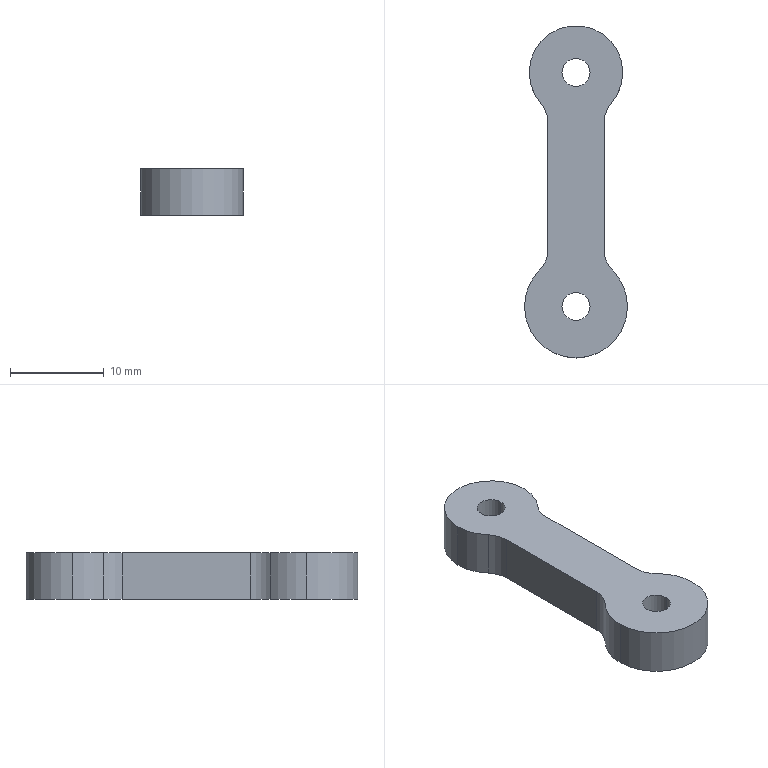Part | SolidWorks | features BaseBody 1 | 1 solid | 18 faces | box 11 x 35.5 x 5 mm | volume 1255 mm3 | cylinder 14 | plane 4 | commonest cylinder face diameters 3 x4 6 x4 10 x3 11 x3
STEP:
#1=CARTESIAN_POINT('',(1.5,25.,5.));
#2=VERTEX_POINT('',#1);
#3=CARTESIAN_POINT('',(1.5,25.,0.));
#4=VERTEX_POINT('',#3);
#5=CARTESIAN_POINT('',(1.5,25.,5.));
#6=DIRECTION('',(0.,0.,-1.));
#7=VECTOR('',#6,1000.);
#8=LINE('',#5,#7);
#9=EDGE_CURVE('',#2,#4,#8,.T.);
#10=ORIENTED_EDGE('',*,*,#9,.F.);
#11=CARTESIAN_POINT('',(-1.5,25.,5.));
#12=VERTEX_POINT('',#11);
#13=CARTESIAN_POINT('',(0.,25.,5.));
#14=DIRECTION('',(0.,0.,1.));
#15=DIRECTION('',(1.,0.,0.));
#16=AXIS2_PLACEMENT_3D('',#13,#14,#15);
#17=CIRCLE('',#16,1.5);
#18=EDGE_CURVE('',#2,#12,#17,.T.);
#19=ORIENTED_EDGE('',*,*,#18,.T.);
#20=CARTESIAN_POINT('',(-1.5,25.,0.));
#21=VERTEX_POINT('',#20);
#22=CARTESIAN_POINT('',(-1.5,25.,5.));
#23=DIRECTION('',(0.,0.,-1.));
#24=VECTOR('',#23,1000.);
#25=LINE('',#22,#24);
#26=EDGE_CURVE('',#12,#21,#25,.T.);
#27=ORIENTED_EDGE('',*,*,#26,.T.);
#28=CARTESIAN_POINT('',(0.,25.,0.));
#29=DIRECTION('',(0.,0.,1.));
#30=DIRECTION('',(1.,0.,0.));
#31=AXIS2_PLACEMENT_3D('',#28,#29,#30);
#32=CIRCLE('',#31,1.5);
#33=EDGE_CURVE('',#4,#21,#32,.T.);
#34=ORIENTED_EDGE('',*,*,#33,.F.);
#35=EDGE_LOOP('',(#10,#19,#27,#34));
#36=FACE_OUTER_BOUND('',#35,.T.);
#37=CARTESIAN_POINT('',(0.,25.,5.));
#38=DIRECTION('',(0.,0.,-1.));
#39=DIRECTION('',(-1.,0.,0.));
#40=AXIS2_PLACEMENT_3D('',#37,#38,#39);
#41=CYLINDRICAL_SURFACE('',#40,1.5);
#42=ADVANCED_FACE('',(#36),#41,.F.);
#43=CARTESIAN_POINT('',(1.5,0.,5.));
#44=VERTEX_POINT('',#43);
#45=CARTESIAN_POINT('',(1.5,0.,0.));
#46=VERTEX_POINT('',#45);
#47=CARTESIAN_POINT('',(1.5,0.,5.));
#48=DIRECTION('',(0.,0.,-1.));
#49=VECTOR('',#48,1000.);
#50=LINE('',#47,#49);
#51=EDGE_CURVE('',#44,#46,#50,.T.);
#52=ORIENTED_EDGE('',*,*,#51,.F.);
#53=CARTESIAN_POINT('',(-1.5,0.,5.));
#54=VERTEX_POINT('',#53);
#55=CARTESIAN_POINT('',(0.,0.,5.));
#56=DIRECTION('',(0.,0.,1.));
#57=DIRECTION('',(1.,0.,0.));
#58=AXIS2_PLACEMENT_3D('',#55,#56,#57);
#59=CIRCLE('',#58,1.5);
#60=EDGE_CURVE('',#44,#54,#59,.T.);
#61=ORIENTED_EDGE('',*,*,#60,.T.);
#62=CARTESIAN_POINT('',(-1.5,0.,0.));
#63=VERTEX_POINT('',#62);
#64=CARTESIAN_POINT('',(-1.5,0.,5.));
#65=DIRECTION('',(0.,0.,-1.));
#66=VECTOR('',#65,1000.);
#67=LINE('',#64,#66);
#68=EDGE_CURVE('',#54,#63,#67,.T.);
#69=ORIENTED_EDGE('',*,*,#68,.T.);
#70=CARTESIAN_POINT('',(0.,0.,0.));
#71=DIRECTION('',(0.,0.,1.));
#72=DIRECTION('',(1.,0.,0.));
#73=AXIS2_PLACEMENT_3D('',#70,#71,#72);
#74=CIRCLE('',#73,1.5);
#75=EDGE_CURVE('',#46,#63,#74,.T.);
#76=ORIENTED_EDGE('',*,*,#75,.F.);
#77=EDGE_LOOP('',(#52,#61,#69,#76));
#78=FACE_OUTER_BOUND('',#77,.T.);
#79=CARTESIAN_POINT('',(0.,0.,5.));
#80=DIRECTION('',(0.,0.,-1.));
#81=DIRECTION('',(-1.,0.,0.));
#82=AXIS2_PLACEMENT_3D('',#79,#80,#81);
#83=CYLINDRICAL_SURFACE('',#82,1.5);
#84=ADVANCED_FACE('',(#78),#83,.F.);
#85=CARTESIAN_POINT('',(-3.,19.708,0.));
#86=VERTEX_POINT('',#85);
#87=CARTESIAN_POINT('',(-3.,6.021,0.));
#88=VERTEX_POINT('',#87);
#89=CARTESIAN_POINT('',(-3.,19.708,0.));
#90=DIRECTION('',(0.,-1.,0.));
#91=VECTOR('',#90,1000.);
#92=LINE('',#89,#91);
#93=EDGE_CURVE('',#86,#88,#92,.T.);
#94=ORIENTED_EDGE('',*,*,#93,.T.);
#95=CARTESIAN_POINT('',(-3.,6.021,5.));
#96=VERTEX_POINT('',#95);
#97=CARTESIAN_POINT('',(-3.,6.021,5.));
#98=DIRECTION('',(0.,0.,-1.));
#99=VECTOR('',#98,1000.);
#100=LINE('',#97,#99);
#101=EDGE_CURVE('',#96,#88,#100,.T.);
#102=ORIENTED_EDGE('',*,*,#101,.F.);
#103=CARTESIAN_POINT('',(-3.,19.708,5.));
#104=VERTEX_POINT('',#103);
#105=CARTESIAN_POINT('',(-3.,19.708,5.));
#106=DIRECTION('',(0.,-1.,0.));
#107=VECTOR('',#106,1000.);
#108=LINE('',#105,#107);
#109=EDGE_CURVE('',#104,#96,#108,.T.);
#110=ORIENTED_EDGE('',*,*,#109,.F.);
#111=CARTESIAN_POINT('',(-3.,19.708,5.));
#112=DIRECTION('',(0.,0.,-1.));
#113=VECTOR('',#112,1000.);
#114=LINE('',#111,#113);
#115=EDGE_CURVE('',#104,#86,#114,.T.);
#116=ORIENTED_EDGE('',*,*,#115,.T.);
#117=EDGE_LOOP('',(#94,#102,#110,#116));
#118=FACE_OUTER_BOUND('',#117,.T.);
#119=CARTESIAN_POINT('',(-3.,19.708,5.));
#120=DIRECTION('',(1.,0.,0.));
#121=DIRECTION('',(0.,1.,0.));
#122=AXIS2_PLACEMENT_3D('',#119,#120,#121);
#123=PLANE('',#122);
#124=ADVANCED_FACE('',(#118),#123,.F.);
#125=CARTESIAN_POINT('',(-3.75,21.693,0.));
#126=VERTEX_POINT('',#125);
#127=CARTESIAN_POINT('',(-6.,19.708,0.));
#128=DIRECTION('',(0.,0.,-1.));
#129=DIRECTION('',(1.,0.,0.));
#130=AXIS2_PLACEMENT_3D('',#127,#128,#129);
#131=CIRCLE('',#130,3.);
#132=EDGE_CURVE('',#126,#86,#131,.T.);
#133=ORIENTED_EDGE('',*,*,#132,.T.);
#134=ORIENTED_EDGE('',*,*,#115,.F.);
#135=CARTESIAN_POINT('',(-3.75,21.693,5.));
#136=VERTEX_POINT('',#135);
#137=CARTESIAN_POINT('',(-6.,19.708,5.));
#138=DIRECTION('',(0.,0.,-1.));
#139=DIRECTION('',(1.,0.,0.));
#140=AXIS2_PLACEMENT_3D('',#137,#138,#139);
#141=CIRCLE('',#140,3.);
#142=EDGE_CURVE('',#136,#104,#141,.T.);
#143=ORIENTED_EDGE('',*,*,#142,.F.);
#144=CARTESIAN_POINT('',(-3.75,21.693,5.));
#145=DIRECTION('',(0.,0.,-1.));
#146=VECTOR('',#145,1000.);
#147=LINE('',#144,#146);
#148=EDGE_CURVE('',#136,#126,#147,.T.);
#149=ORIENTED_EDGE('',*,*,#148,.T.);
#150=EDGE_LOOP('',(#133,#134,#143,#149));
#151=FACE_OUTER_BOUND('',#150,.T.);
#152=CARTESIAN_POINT('',(-6.,19.708,5.));
#153=DIRECTION('',(0.,0.,-1.));
#154=DIRECTION('',(-1.,0.,0.));
#155=AXIS2_PLACEMENT_3D('',#152,#153,#154);
#156=CYLINDRICAL_SURFACE('',#155,3.);
#157=ADVANCED_FACE('',(#151),#156,.F.);
#158=CARTESIAN_POINT('',(5.,25.,5.));
#159=VERTEX_POINT('',#158);
#160=CARTESIAN_POINT('',(5.,25.,0.));
#161=VERTEX_POINT('',#160);
#162=CARTESIAN_POINT('',(5.,25.,5.));
#163=DIRECTION('',(0.,0.,-1.));
#164=VECTOR('',#163,1000.);
#165=LINE('',#162,#164);
#166=EDGE_CURVE('',#159,#161,#165,.T.);
#167=ORIENTED_EDGE('',*,*,#166,.F.);
#168=CARTESIAN_POINT('',(3.75,21.693,5.));
#169=VERTEX_POINT('',#168);
#170=CARTESIAN_POINT('',(0.,25.,5.));
#171=DIRECTION('',(0.,0.,1.));
#172=DIRECTION('',(1.,0.,0.));
#173=AXIS2_PLACEMENT_3D('',#170,#171,#172);
#174=CIRCLE('',#173,5.);
#175=EDGE_CURVE('',#169,#159,#174,.T.);
#176=ORIENTED_EDGE('',*,*,#175,.F.);
#177=CARTESIAN_POINT('',(3.75,21.693,0.));
#178=VERTEX_POINT('',#177);
#179=CARTESIAN_POINT('',(3.75,21.693,5.));
#180=DIRECTION('',(0.,0.,-1.));
#181=VECTOR('',#180,1000.);
#182=LINE('',#179,#181);
#183=EDGE_CURVE('',#169,#178,#182,.T.);
#184=ORIENTED_EDGE('',*,*,#183,.T.);
#185=CARTESIAN_POINT('',(0.,25.,0.));
#186=DIRECTION('',(0.,0.,1.));
#187=DIRECTION('',(1.,0.,0.));
#188=AXIS2_PLACEMENT_3D('',#185,#186,#187);
#189=CIRCLE('',#188,5.);
#190=EDGE_CURVE('',#178,#161,#189,.T.);
#191=ORIENTED_EDGE('',*,*,#190,.T.);
#192=EDGE_LOOP('',(#167,#176,#184,#191));
#193=FACE_OUTER_BOUND('',#192,.T.);
#194=CARTESIAN_POINT('',(0.,25.,5.));
#195=DIRECTION('',(0.,0.,-1.));
#196=DIRECTION('',(-1.,0.,0.));
#197=AXIS2_PLACEMENT_3D('',#194,#195,#196);
#198=CYLINDRICAL_SURFACE('',#197,5.);
#199=ADVANCED_FACE('',(#193),#198,.T.);
#200=CARTESIAN_POINT('',(3.,19.708,0.));
#201=VERTEX_POINT('',#200);
#202=CARTESIAN_POINT('',(6.,19.708,0.));
#203=DIRECTION('',(0.,0.,-1.));
#204=DIRECTION('',(-1.,0.,0.));
#205=AXIS2_PLACEMENT_3D('',#202,#203,#204);
#206=CIRCLE('',#205,3.);
#207=EDGE_CURVE('',#201,#178,#206,.T.);
#208=ORIENTED_EDGE('',*,*,#207,.T.);
#209=ORIENTED_EDGE('',*,*,#183,.F.);
#210=CARTESIAN_POINT('',(3.,19.708,5.));
#211=VERTEX_POINT('',#210);
#212=CARTESIAN_POINT('',(6.,19.708,5.));
#213=DIRECTION('',(0.,0.,-1.));
#214=DIRECTION('',(-1.,0.,0.));
#215=AXIS2_PLACEMENT_3D('',#212,#213,#214);
#216=CIRCLE('',#215,3.);
#217=EDGE_CURVE('',#211,#169,#216,.T.);
#218=ORIENTED_EDGE('',*,*,#217,.F.);
#219=CARTESIAN_POINT('',(3.,19.708,5.));
#220=DIRECTION('',(0.,0.,-1.));
#221=VECTOR('',#220,1000.);
#222=LINE('',#219,#221);
#223=EDGE_CURVE('',#211,#201,#222,.T.);
#224=ORIENTED_EDGE('',*,*,#223,.T.);
#225=EDGE_LOOP('',(#208,#209,#218,#224));
#226=FACE_OUTER_BOUND('',#225,.T.);
#227=CARTESIAN_POINT('',(6.,19.708,5.));
#228=DIRECTION('',(0.,0.,-1.));
#229=DIRECTION('',(-1.,0.,0.));
#230=AXIS2_PLACEMENT_3D('',#227,#228,#229);
#231=CYLINDRICAL_SURFACE('',#230,3.);
#232=ADVANCED_FACE('',(#226),#231,.F.);
#233=CARTESIAN_POINT('',(3.,6.021,0.));
#234=VERTEX_POINT('',#233);
#235=CARTESIAN_POINT('',(3.,19.708,0.));
#236=DIRECTION('',(0.,1.,0.));
#237=VECTOR('',#236,1000.);
#238=LINE('',#235,#237);
#239=EDGE_CURVE('',#234,#201,#238,.T.);
#240=ORIENTED_EDGE('',*,*,#239,.T.);
#241=ORIENTED_EDGE('',*,*,#223,.F.);
#242=CARTESIAN_POINT('',(3.,6.021,5.));
#243=VERTEX_POINT('',#242);
#244=CARTESIAN_POINT('',(3.,19.708,5.));
#245=DIRECTION('',(0.,1.,0.));
#246=VECTOR('',#245,1000.);
#247=LINE('',#244,#246);
#248=EDGE_CURVE('',#243,#211,#247,.T.);
#249=ORIENTED_EDGE('',*,*,#248,.F.);
#250=CARTESIAN_POINT('',(3.,6.021,5.));
#251=DIRECTION('',(0.,0.,-1.));
#252=VECTOR('',#251,1000.);
#253=LINE('',#250,#252);
#254=EDGE_CURVE('',#243,#234,#253,.T.);
#255=ORIENTED_EDGE('',*,*,#254,.T.);
#256=EDGE_LOOP('',(#240,#241,#249,#255));
#257=FACE_OUTER_BOUND('',#256,.T.);
#258=CARTESIAN_POINT('',(3.,19.708,5.));
#259=DIRECTION('',(-1.,0.,0.));
#260=DIRECTION('',(0.,1.,0.));
#261=AXIS2_PLACEMENT_3D('',#258,#259,#260);
#262=PLANE('',#261);
#263=ADVANCED_FACE('',(#257),#262,.F.);
#264=CARTESIAN_POINT('',(3.882,3.896,0.));
#265=VERTEX_POINT('',#264);
#266=CARTESIAN_POINT('',(6.,6.021,0.));
#267=DIRECTION('',(0.,0.,-1.));
#268=DIRECTION('',(-1.,0.,0.));
#269=AXIS2_PLACEMENT_3D('',#266,#267,#268);
#270=CIRCLE('',#269,3.);
#271=EDGE_CURVE('',#265,#234,#270,.T.);
#272=ORIENTED_EDGE('',*,*,#271,.T.);
#273=ORIENTED_EDGE('',*,*,#254,.F.);
#274=CARTESIAN_POINT('',(3.882,3.896,5.));
#275=VERTEX_POINT('',#274);
#276=CARTESIAN_POINT('',(6.,6.021,5.));
#277=DIRECTION('',(0.,0.,-1.));
#278=DIRECTION('',(-1.,0.,0.));
#279=AXIS2_PLACEMENT_3D('',#276,#277,#278);
#280=CIRCLE('',#279,3.);
#281=EDGE_CURVE('',#275,#243,#280,.T.);
#282=ORIENTED_EDGE('',*,*,#281,.F.);
#283=CARTESIAN_POINT('',(3.882,3.896,5.));
#284=DIRECTION('',(0.,0.,-1.));
#285=VECTOR('',#284,1000.);
#286=LINE('',#283,#285);
#287=EDGE_CURVE('',#275,#265,#286,.T.);
#288=ORIENTED_EDGE('',*,*,#287,.T.);
#289=EDGE_LOOP('',(#272,#273,#282,#288));
#290=FACE_OUTER_BOUND('',#289,.T.);
#291=CARTESIAN_POINT('',(6.,6.021,5.));
#292=DIRECTION('',(0.,0.,-1.));
#293=DIRECTION('',(-1.,0.,0.));
#294=AXIS2_PLACEMENT_3D('',#291,#292,#293);
#295=CYLINDRICAL_SURFACE('',#294,3.);
#296=ADVANCED_FACE('',(#290),#295,.F.);
#297=CARTESIAN_POINT('',(-5.5,0.,5.));
#298=VERTEX_POINT('',#297);
#299=CARTESIAN_POINT('',(-5.5,0.,0.));
#300=VERTEX_POINT('',#299);
#301=CARTESIAN_POINT('',(-5.5,0.,5.));
#302=DIRECTION('',(0.,0.,-1.));
#303=VECTOR('',#302,1000.);
#304=LINE('',#301,#303);
#305=EDGE_CURVE('',#298,#300,#304,.T.);
#306=ORIENTED_EDGE('',*,*,#305,.F.);
#307=CARTESIAN_POINT('',(-3.882,3.896,5.));
#308=VERTEX_POINT('',#307);
#309=CARTESIAN_POINT('',(0.,0.,5.));
#310=DIRECTION('',(0.,0.,1.));
#311=DIRECTION('',(1.,0.,0.));
#312=AXIS2_PLACEMENT_3D('',#309,#310,#311);
#313=CIRCLE('',#312,5.5);
#314=EDGE_CURVE('',#308,#298,#313,.T.);
#315=ORIENTED_EDGE('',*,*,#314,.F.);
#316=CARTESIAN_POINT('',(-3.882,3.896,0.));
#317=VERTEX_POINT('',#316);
#318=CARTESIAN_POINT('',(-3.882,3.896,5.));
#319=DIRECTION('',(0.,0.,-1.));
#320=VECTOR('',#319,1000.);
#321=LINE('',#318,#320);
#322=EDGE_CURVE('',#308,#317,#321,.T.);
#323=ORIENTED_EDGE('',*,*,#322,.T.);
#324=CARTESIAN_POINT('',(0.,0.,0.));
#325=DIRECTION('',(0.,0.,1.));
#326=DIRECTION('',(1.,0.,0.));
#327=AXIS2_PLACEMENT_3D('',#324,#325,#326);
#328=CIRCLE('',#327,5.5);
#329=EDGE_CURVE('',#317,#300,#328,.T.);
#330=ORIENTED_EDGE('',*,*,#329,.T.);
#331=EDGE_LOOP('',(#306,#315,#323,#330));
#332=FACE_OUTER_BOUND('',#331,.T.);
#333=CARTESIAN_POINT('',(0.,0.,5.));
#334=DIRECTION('',(0.,0.,-1.));
#335=DIRECTION('',(-1.,0.,0.));
#336=AXIS2_PLACEMENT_3D('',#333,#334,#335);
#337=CYLINDRICAL_SURFACE('',#336,5.5);
#338=ADVANCED_FACE('',(#332),#337,.T.);
#339=CARTESIAN_POINT('',(-6.,6.021,0.));
#340=DIRECTION('',(0.,0.,-1.));
#341=DIRECTION('',(1.,0.,0.));
#342=AXIS2_PLACEMENT_3D('',#339,#340,#341);
#343=CIRCLE('',#342,3.);
#344=EDGE_CURVE('',#88,#317,#343,.T.);
#345=ORIENTED_EDGE('',*,*,#344,.T.);
#346=ORIENTED_EDGE('',*,*,#322,.F.);
#347=CARTESIAN_POINT('',(-6.,6.021,5.));
#348=DIRECTION('',(0.,0.,-1.));
#349=DIRECTION('',(1.,0.,0.));
#350=AXIS2_PLACEMENT_3D('',#347,#348,#349);
#351=CIRCLE('',#350,3.);
#352=EDGE_CURVE('',#96,#308,#351,.T.);
#353=ORIENTED_EDGE('',*,*,#352,.F.);
#354=ORIENTED_EDGE('',*,*,#101,.T.);
#355=EDGE_LOOP('',(#345,#346,#353,#354));
#356=FACE_OUTER_BOUND('',#355,.T.);
#357=CARTESIAN_POINT('',(-6.,6.021,5.));
#358=DIRECTION('',(0.,0.,-1.));
#359=DIRECTION('',(-1.,0.,0.));
#360=AXIS2_PLACEMENT_3D('',#357,#358,#359);
#361=CYLINDRICAL_SURFACE('',#360,3.);
#362=ADVANCED_FACE('',(#356),#361,.F.);
#363=CARTESIAN_POINT('',(0.,25.,0.));
#364=DIRECTION('',(0.,0.,1.));
#365=DIRECTION('',(1.,0.,0.));
#366=AXIS2_PLACEMENT_3D('',#363,#364,#365);
#367=CIRCLE('',#366,1.5);
#368=EDGE_CURVE('',#21,#4,#367,.T.);
#369=ORIENTED_EDGE('',*,*,#368,.T.);
#370=ORIENTED_EDGE('',*,*,#33,.T.);
#371=EDGE_LOOP('',(#369,#370));
#372=FACE_BOUND('',#371,.T.);
#373=CARTESIAN_POINT('',(0.,0.,0.));
#374=DIRECTION('',(0.,0.,1.));
#375=DIRECTION('',(1.,0.,0.));
#376=AXIS2_PLACEMENT_3D('',#373,#374,#375);
#377=CIRCLE('',#376,1.5);
#378=EDGE_CURVE('',#63,#46,#377,.T.);
#379=ORIENTED_EDGE('',*,*,#378,.T.);
#380=ORIENTED_EDGE('',*,*,#75,.T.);
#381=EDGE_LOOP('',(#379,#380));
#382=FACE_BOUND('',#381,.T.);
#383=ORIENTED_EDGE('',*,*,#344,.F.);
#384=ORIENTED_EDGE('',*,*,#93,.F.);
#385=ORIENTED_EDGE('',*,*,#132,.F.);
#386=CARTESIAN_POINT('',(-5.,25.,0.));
#387=VERTEX_POINT('',#386);
#388=CARTESIAN_POINT('',(0.,25.,0.));
#389=DIRECTION('',(0.,0.,1.));
#390=DIRECTION('',(1.,0.,0.));
#391=AXIS2_PLACEMENT_3D('',#388,#389,#390);
#392=CIRCLE('',#391,5.);
#393=EDGE_CURVE('',#387,#126,#392,.T.);
#394=ORIENTED_EDGE('',*,*,#393,.F.);
#395=CARTESIAN_POINT('',(0.,25.,0.));
#396=DIRECTION('',(0.,0.,1.));
#397=DIRECTION('',(1.,0.,0.));
#398=AXIS2_PLACEMENT_3D('',#395,#396,#397);
#399=CIRCLE('',#398,5.);
#400=EDGE_CURVE('',#161,#387,#399,.T.);
#401=ORIENTED_EDGE('',*,*,#400,.F.);
#402=ORIENTED_EDGE('',*,*,#190,.F.);
#403=ORIENTED_EDGE('',*,*,#207,.F.);
#404=ORIENTED_EDGE('',*,*,#239,.F.);
#405=ORIENTED_EDGE('',*,*,#271,.F.);
#406=CARTESIAN_POINT('',(5.5,0.,0.));
#407=VERTEX_POINT('',#406);
#408=CARTESIAN_POINT('',(0.,0.,0.));
#409=DIRECTION('',(0.,0.,1.));
#410=DIRECTION('',(1.,0.,0.));
#411=AXIS2_PLACEMENT_3D('',#408,#409,#410);
#412=CIRCLE('',#411,5.5);
#413=EDGE_CURVE('',#407,#265,#412,.T.);
#414=ORIENTED_EDGE('',*,*,#413,.F.);
#415=CARTESIAN_POINT('',(0.,0.,0.));
#416=DIRECTION('',(0.,0.,1.));
#417=DIRECTION('',(1.,0.,0.));
#418=AXIS2_PLACEMENT_3D('',#415,#416,#417);
#419=CIRCLE('',#418,5.5);
#420=EDGE_CURVE('',#300,#407,#419,.T.);
#421=ORIENTED_EDGE('',*,*,#420,.F.);
#422=ORIENTED_EDGE('',*,*,#329,.F.);
#423=EDGE_LOOP('',(#383,#384,#385,#394,#401,#402,#403,#404,#405,#414,#421,#422));
#424=FACE_OUTER_BOUND('',#423,.T.);
#425=CARTESIAN_POINT('',(-6.,6.021,0.));
#426=DIRECTION('',(0.,0.,1.));
#427=DIRECTION('',(1.,0.,0.));
#428=AXIS2_PLACEMENT_3D('',#425,#426,#427);
#429=PLANE('',#428);
#430=ADVANCED_FACE('',(#372,#382,#424),#429,.F.);
#431=CARTESIAN_POINT('',(0.,25.,5.));
#432=DIRECTION('',(0.,0.,1.));
#433=DIRECTION('',(1.,0.,0.));
#434=AXIS2_PLACEMENT_3D('',#431,#432,#433);
#435=CIRCLE('',#434,1.5);
#436=EDGE_CURVE('',#12,#2,#435,.T.);
#437=ORIENTED_EDGE('',*,*,#436,.F.);
#438=ORIENTED_EDGE('',*,*,#18,.F.);
#439=EDGE_LOOP('',(#437,#438));
#440=FACE_BOUND('',#439,.T.);
#441=CARTESIAN_POINT('',(0.,0.,5.));
#442=DIRECTION('',(0.,0.,1.));
#443=DIRECTION('',(1.,0.,0.));
#444=AXIS2_PLACEMENT_3D('',#441,#442,#443);
#445=CIRCLE('',#444,1.5);
#446=EDGE_CURVE('',#54,#44,#445,.T.);
#447=ORIENTED_EDGE('',*,*,#446,.F.);
#448=ORIENTED_EDGE('',*,*,#60,.F.);
#449=EDGE_LOOP('',(#447,#448));
#450=FACE_BOUND('',#449,.T.);
#451=ORIENTED_EDGE('',*,*,#352,.T.);
#452=ORIENTED_EDGE('',*,*,#314,.T.);
#453=CARTESIAN_POINT('',(5.5,0.,5.));
#454=VERTEX_POINT('',#453);
#455=CARTESIAN_POINT('',(0.,0.,5.));
#456=DIRECTION('',(0.,0.,1.));
#457=DIRECTION('',(1.,0.,0.));
#458=AXIS2_PLACEMENT_3D('',#455,#456,#457);
#459=CIRCLE('',#458,5.5);
#460=EDGE_CURVE('',#298,#454,#459,.T.);
#461=ORIENTED_EDGE('',*,*,#460,.T.);
#462=CARTESIAN_POINT('',(0.,0.,5.));
#463=DIRECTION('',(0.,0.,1.));
#464=DIRECTION('',(1.,0.,0.));
#465=AXIS2_PLACEMENT_3D('',#462,#463,#464);
#466=CIRCLE('',#465,5.5);
#467=EDGE_CURVE('',#454,#275,#466,.T.);
#468=ORIENTED_EDGE('',*,*,#467,.T.);
#469=ORIENTED_EDGE('',*,*,#281,.T.);
#470=ORIENTED_EDGE('',*,*,#248,.T.);
#471=ORIENTED_EDGE('',*,*,#217,.T.);
#472=ORIENTED_EDGE('',*,*,#175,.T.);
#473=CARTESIAN_POINT('',(-5.,25.,5.));
#474=VERTEX_POINT('',#473);
#475=CARTESIAN_POINT('',(0.,25.,5.));
#476=DIRECTION('',(0.,0.,1.));
#477=DIRECTION('',(1.,0.,0.));
#478=AXIS2_PLACEMENT_3D('',#475,#476,#477);
#479=CIRCLE('',#478,5.);
#480=EDGE_CURVE('',#159,#474,#479,.T.);
#481=ORIENTED_EDGE('',*,*,#480,.T.);
#482=CARTESIAN_POINT('',(0.,25.,5.));
#483=DIRECTION('',(0.,0.,1.));
#484=DIRECTION('',(1.,0.,0.));
#485=AXIS2_PLACEMENT_3D('',#482,#483,#484);
#486=CIRCLE('',#485,5.);
#487=EDGE_CURVE('',#474,#136,#486,.T.);
#488=ORIENTED_EDGE('',*,*,#487,.T.);
#489=ORIENTED_EDGE('',*,*,#142,.T.);
#490=ORIENTED_EDGE('',*,*,#109,.T.);
#491=EDGE_LOOP('',(#451,#452,#461,#468,#469,#470,#471,#472,#481,#488,#489,#490));
#492=FACE_OUTER_BOUND('',#491,.T.);
#493=CARTESIAN_POINT('',(-6.,6.021,5.));
#494=DIRECTION('',(0.,0.,1.));
#495=DIRECTION('',(1.,0.,0.));
#496=AXIS2_PLACEMENT_3D('',#493,#494,#495);
#497=PLANE('',#496);
#498=ADVANCED_FACE('',(#440,#450,#492),#497,.T.);
#499=CARTESIAN_POINT('',(5.5,0.,5.));
#500=DIRECTION('',(0.,0.,-1.));
#501=VECTOR('',#500,1000.);
#502=LINE('',#499,#501);
#503=EDGE_CURVE('',#454,#407,#502,.T.);
#504=ORIENTED_EDGE('',*,*,#503,.F.);
#505=ORIENTED_EDGE('',*,*,#460,.F.);
#506=ORIENTED_EDGE('',*,*,#305,.T.);
#507=ORIENTED_EDGE('',*,*,#420,.T.);
#508=EDGE_LOOP('',(#504,#505,#506,#507));
#509=FACE_OUTER_BOUND('',#508,.T.);
#510=CARTESIAN_POINT('',(0.,0.,5.));
#511=DIRECTION('',(0.,0.,-1.));
#512=DIRECTION('',(-1.,0.,0.));
#513=AXIS2_PLACEMENT_3D('',#510,#511,#512);
#514=CYLINDRICAL_SURFACE('',#513,5.5);
#515=ADVANCED_FACE('',(#509),#514,.T.);
#516=ORIENTED_EDGE('',*,*,#467,.F.);
#517=ORIENTED_EDGE('',*,*,#503,.T.);
#518=ORIENTED_EDGE('',*,*,#413,.T.);
#519=ORIENTED_EDGE('',*,*,#287,.F.);
#520=EDGE_LOOP('',(#516,#517,#518,#519));
#521=FACE_OUTER_BOUND('',#520,.T.);
#522=CARTESIAN_POINT('',(0.,0.,5.));
#523=DIRECTION('',(0.,0.,-1.));
#524=DIRECTION('',(-1.,0.,0.));
#525=AXIS2_PLACEMENT_3D('',#522,#523,#524);
#526=CYLINDRICAL_SURFACE('',#525,5.5);
#527=ADVANCED_FACE('',(#521),#526,.T.);
#528=ORIENTED_EDGE('',*,*,#487,.F.);
#529=CARTESIAN_POINT('',(-5.,25.,5.));
#530=DIRECTION('',(0.,0.,-1.));
#531=VECTOR('',#530,1000.);
#532=LINE('',#529,#531);
#533=EDGE_CURVE('',#474,#387,#532,.T.);
#534=ORIENTED_EDGE('',*,*,#533,.T.);
#535=ORIENTED_EDGE('',*,*,#393,.T.);
#536=ORIENTED_EDGE('',*,*,#148,.F.);
#537=EDGE_LOOP('',(#528,#534,#535,#536));
#538=FACE_OUTER_BOUND('',#537,.T.);
#539=CARTESIAN_POINT('',(0.,25.,5.));
#540=DIRECTION('',(0.,0.,-1.));
#541=DIRECTION('',(-1.,0.,0.));
#542=AXIS2_PLACEMENT_3D('',#539,#540,#541);
#543=CYLINDRICAL_SURFACE('',#542,5.);
#544=ADVANCED_FACE('',(#538),#543,.T.);
#545=ORIENTED_EDGE('',*,*,#480,.F.);
#546=ORIENTED_EDGE('',*,*,#166,.T.);
#547=ORIENTED_EDGE('',*,*,#400,.T.);
#548=ORIENTED_EDGE('',*,*,#533,.F.);
#549=EDGE_LOOP('',(#545,#546,#547,#548));
#550=FACE_OUTER_BOUND('',#549,.T.);
#551=CARTESIAN_POINT('',(0.,25.,5.));
#552=DIRECTION('',(0.,0.,-1.));
#553=DIRECTION('',(-1.,0.,0.));
#554=AXIS2_PLACEMENT_3D('',#551,#552,#553);
#555=CYLINDRICAL_SURFACE('',#554,5.);
#556=ADVANCED_FACE('',(#550),#555,.T.);
#557=ORIENTED_EDGE('',*,*,#446,.T.);
#558=ORIENTED_EDGE('',*,*,#51,.T.);
#559=ORIENTED_EDGE('',*,*,#378,.F.);
#560=ORIENTED_EDGE('',*,*,#68,.F.);
#561=EDGE_LOOP('',(#557,#558,#559,#560));
#562=FACE_OUTER_BOUND('',#561,.T.);
#563=CARTESIAN_POINT('',(0.,0.,5.));
#564=DIRECTION('',(0.,0.,-1.));
#565=DIRECTION('',(-1.,0.,0.));
#566=AXIS2_PLACEMENT_3D('',#563,#564,#565);
#567=CYLINDRICAL_SURFACE('',#566,1.5);
#568=ADVANCED_FACE('',(#562),#567,.F.);
#569=ORIENTED_EDGE('',*,*,#436,.T.);
#570=ORIENTED_EDGE('',*,*,#9,.T.);
#571=ORIENTED_EDGE('',*,*,#368,.F.);
#572=ORIENTED_EDGE('',*,*,#26,.F.);
#573=EDGE_LOOP('',(#569,#570,#571,#572));
#574=FACE_OUTER_BOUND('',#573,.T.);
#575=CARTESIAN_POINT('',(0.,25.,5.));
#576=DIRECTION('',(0.,0.,-1.));
#577=DIRECTION('',(-1.,0.,0.));
#578=AXIS2_PLACEMENT_3D('',#575,#576,#577);
#579=CYLINDRICAL_SURFACE('',#578,1.5);
#580=ADVANCED_FACE('',(#574),#579,.F.);
#581=CLOSED_SHELL('',(#42,#84,#124,#157,#199,#232,#263,#296,#338,#362,#430,#498,#515,#527,#544,#556,#568,#580));
#582=MANIFOLD_SOLID_BREP('',#581);
#583=CARTESIAN_POINT('',(0.,0.,0.));
#584=DIRECTION('',(0.,0.,1.));
#585=DIRECTION('',(1.,0.,0.));
#586=AXIS2_PLACEMENT_3D('',#583,#584,#585);
#587=(LENGTH_UNIT()NAMED_UNIT(*)SI_UNIT(.MILLI.,.METRE.));
#588=UNCERTAINTY_MEASURE_WITH_UNIT(LENGTH_MEASURE(0.00001),#587,'','');
#589=(NAMED_UNIT(*)PLANE_ANGLE_UNIT()SI_UNIT($,.RADIAN.));
#590=(NAMED_UNIT(*)SI_UNIT($,.STERADIAN.)SOLID_ANGLE_UNIT());
#591=(GEOMETRIC_REPRESENTATION_CONTEXT(3)GLOBAL_UNCERTAINTY_ASSIGNED_CONTEXT((#588))GLOBAL_UNIT_ASSIGNED_CONTEXT((#587,#589,#590))REPRESENTATION_CONTEXT('',''));
#592=ADVANCED_BREP_SHAPE_REPRESENTATION('',(#582,#586),#591);